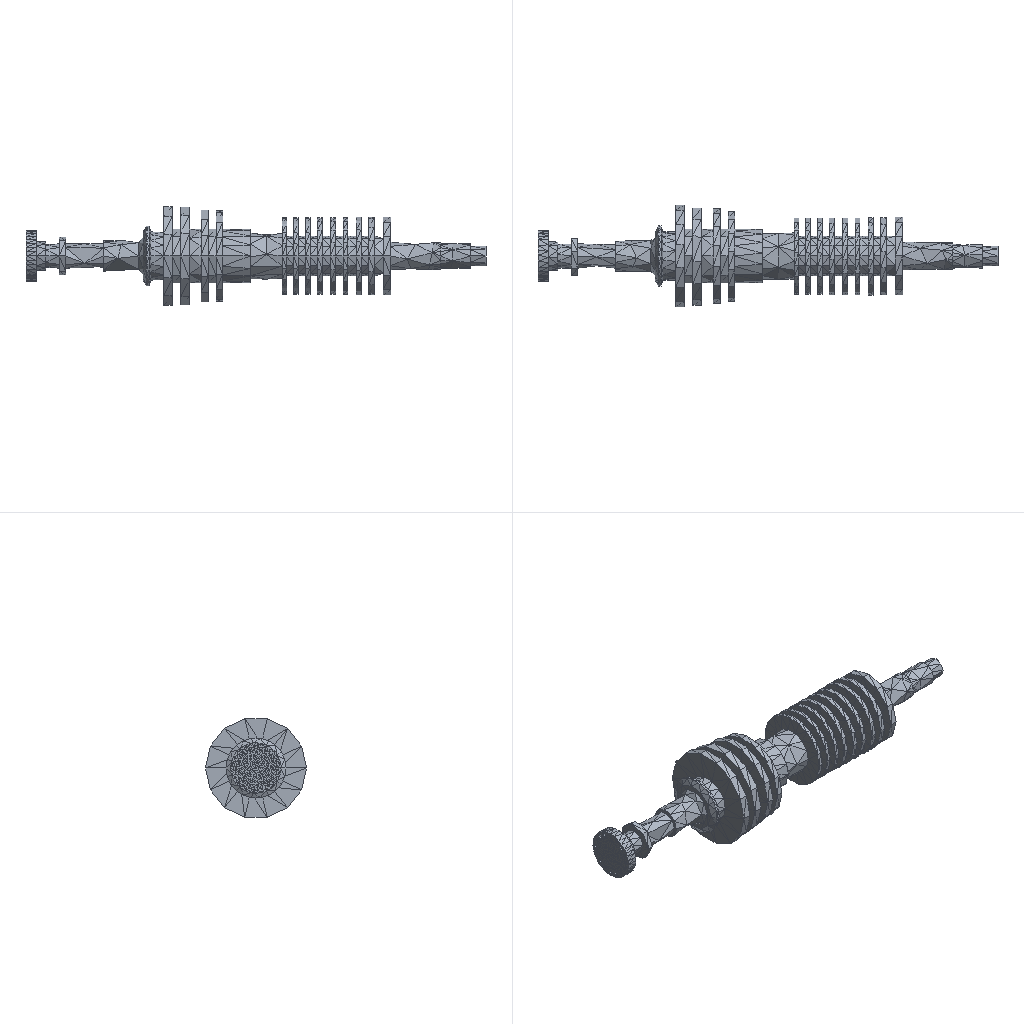Simulation study | ansys workbench
Ansys APDL input file, long lists of numbers shortened:
/batch
/config,noeldb,1     ! force off writing results to database
*get,_wallstrt,active,,time,wall
! ANSYS input file written by Workbench version 2022 R1
! File used for geometry attach:
/title,_______--__ (C5)
! ****** Begin Custom Load Command Snippet ******
/COM, ACT Extensions:
/COM,     LSDYNA, 2021.1
/COM,
! ****** End   Custom Load Command Snippet ******
*DIM,_wb_ProjectScratch_dir,string,248
_wb_ProjectScratch_dir(1) = ''
*DIM,_wb_SolverFiles_dir,string,248
_wb_SolverFiles_dir(1) = ''
*DIM,_wb_userfiles_dir,string,248
_wb_userfiles_dir(1) = ''
/com,--- Data in consistent NMM units. See Solving Units in the help system for more information.
/units,MPA
/nopr
/wb,file,start              !  signify a WB generated input file
/prep7
! Turn off shape checking because checks already performed inside WB mesher.
! See help system for more information.
SHPP,OFF,,NOWARN
/nolist
etcon,set             ! allow ANSYS to choose best KEYOP's for 180x elements, resets any applicable keyopt to MAPDL defaults
/com,*********** Nodes for the whole assembly ***********
nblock,3,,19310
(1i9,3e20.9e3)
        1     4.906201621E+04    -3.060000000E+02     1.550000000E+03
! (17554 more lines like these left out)
-1
/com,*********** Nodes for all Remote Points ***********
nblock,3
(1i9,3e20.9e3)
    17556     4.888853330E+04     3.865628677E-15     1.549999997E+03
-1
/wb,elem,start            !  set before creation of elements
/com,*********** Elements for Body 1 "_____+115mm\_____" ***********
et,1,187
eblock,19,solid,,9763
(19i9)
        1        1        1        1        0        0        0        0       10        0        1     2257     2779     2330     2541    15734    16136    15725    15727
! (19525 more lines like these left out)
-1
/wb,elem,end               !  done creating elements
/com,*********** Send User Defined Coordinate System(s) ***********
csys,0
toffst,273.15,  ! Temperature offset from absolute zero
/com,*********** Set Reference Temperature ***********
tref,22.
/wb,mat,start              !  starting to send materials
/com,*********** Send Materials ***********
Temperature = 'TEMP' ! Temperature
MP,DENS,1,7.85e-09,	! tonne mm^-3
MP,ALPX,1,1.2e-05,	! C^-1
MP,C,1,434000000,	! mm^2 s^-2 C^-1
MP,KXX,1,60.5,	! tonne mm s^-3 C^-1
MP,RSVX,1,0.00017,	! ohm mm
MP,EX,1,200000,	! tonne s^-2 mm^-1
MP,NUXY,1,0.3,
MP,MURX,1,10000,
/wb,mat,end                !  done sending materials
!************************* Model Summary ********************
!_____+115mm\_____,	结构钢,	matid,	1
!************************* End Model Summary ********************
! get the diagonal of the bounding box. Needed later for other things
*get,_xmin,node,,mnloc,x
*get,_ymin,node,,mnloc,y
*get,_zmin,node,,mnloc,z
*get,_xmax,node,,mxloc,x
*get,_ymax,node,,mxloc,y
*get,_zmax,node,,mxloc,z
_ASMDIAG=(_xmax-_xmin)*(_xmax-_xmin)+(_ymax-_ymin)*(_ymax-_ymin)+(_zmax-_zmin)*(_zmax-_zmin)
_ASMDIAG=SQRT(_ASMDIAG)
/wb,contact,start          !  starting to send contact
/wb,contact,end            !  done creating contacts
/golist
/wb,load,start             !  starting to send loads
/com,*********** Fixed Supports ***********
CMBLOCK,_FIXEDSU,NODE,      114
(8i10)
       876       877       878       879       880       881       882       883
! (14 more lines like these left out)
cmsel,s,_FIXEDSU
d,all,all
nsel,all
/com,*********** Create Remote Point "内部远程点" ***********
! -------- Remote Point Used by "力矩" --------
*set,tid,3
*set,cid,2
et,cid,174
et,tid,170
keyo,tid,2,1               ! Don't fix the pilot node
keyo,tid,4,0               ! Activate all DOF's due to large deformation
keyo,cid,12,5              ! Bonded Contact
keyo,cid,4,1               ! Deformable RBE3 style load
keyo,cid,2,2               ! MPC style contact
eblock,10,,,154
(15i9)
    14157        2        2        2        0      857      858     2037     2037     7802     7809     2037     7805
! (153 more lines like these left out)
-1
*set,_npilot,17556
_npilot33=_npilot
type,tid
mat ,cid
real,cid
tshape,pilo
en,14311,_npilot
tshape
/com,*********** Construct Moment Using Remote Attachment ***********
/gst,on,on
fini
*get,_numnode,node,0,count
*get,_numelem,elem,0,count
*get, _MAXELEMNUM, elem, 0, NUM, MAX
*get, _MAXNODENUM, node, 0, NUM, MAX
*get, _MAXELEMTYPE, etyp, 0, NUM, MAX
*get, _MAXREALCONST, real, 0, NUM, MAX
/go
/wb,load,end               !  done creating loads
/com,--- Number of total nodes = %_numnode%
/com,--- Number of contact elements = 154
/com,--- Number of spring elements = 0
/com,--- Number of bearing elements = 0
/com,--- Number of solid elements = 9763
/com,--- Number of condensed parts = 0
/com,--- Number of total elements = %_numelem%
*get,_wallbsol,active,,time,wall
/com,****************************************************************************
/com,*************************    SOLUTION       ********************************
/com,****************************************************************************
/solu
antype,4                   ! transient analysis
nlgeom,on                  ! Turn on Large Deformation Effects
kbc,1                      ! stepped BC's
_thickRatio=  1     ! Ratio of thick parts in the model
eqsl,pcg,1e-8,,,,,,1
cntr,print,1               ! print out contact info and also make no initial contact an error
dmpoption,emat,no             ! Don't combine emat file for DANSYS
dmpoption,esav,no             ! Don't combine esav file for DANSYS
trnopt,full,,,,,hht        ! HHT time integration method
tintp, mosp			! Choose transient integration settings for moderate speed application
nldiag,cont,iter           ! print out contact info each equilibrium iteration
rescontrol,define,last,last,,dele	   ! Program Controlled
/com,****************************************************
/com,******************* SOLVE FOR LS 1 OF 1 ****************
nsel,s,node,,17556
f,all,mx,150.
f,all,my,0.
f,all,mz,0.
nsel,all
/nopr
/gopr
autots,on                   ! User turned on automatic time stepping
deltim,20,20,20,OFF
time,20.
timint,on                  ! Turn on time integration effects
outres,erase
outres,all,none
outres,nsol,all,
outres,rsol,all
outres,eangl,all
outres,etmp,all
outres,veng,all
outres,strs,all,
outres,epel,all,
outres,eppl,all,
outres,cont,all,
outres,v,all,
outres,a,all,
! *********** WB SOLVE COMMAND ***********
! check interactive state
*get,ANSINTER_,active,,int
*if,ANSINTER_,ne,0,then
/eof
*endif
solve
/com *************** Write FE CONNECTORS *********
CEWRITE,file,ce,,INTE
/com,****************************************************
/com,*************** FINISHED SOLVE FOR LS 1 *************
*get,_wallasol,active,,time,wall
/nopr
*get,_numnode,node,0,count
*get,_numelem,elem,0,count
*get, _MAXELEMNUM, elem, 0, NUM, MAX
*get, _MAXNODENUM, node, 0, NUM, MAX,,,INTERNAL
*get, _MAXELEMTYPE, etyp, 0, NUM, MAX
*get, _MAXREALCONST, real, 0, NUM, MAX
/gopr
*get,_PCGITER,active,,solu,cgiter
/post1
xmlo,ENCODING,ISO-8859-1
xmlo,parm
/xml,parm,xml
fini
/gopr
*get,_walldone,active,,time,wall
_preptime=(_wallbsol-_wallstrt)*3600
_solvtime=(_wallasol-_wallbsol)*3600
_posttime=(_walldone-_wallasol)*3600
_totaltim=(_walldone-_wallstrt)*3600
*get,_dlbratio,active,0,solu,dlbr
*get,_combtime,active,0,solu,comb
*get,_ssmode,active,0,solu,ssmm
*get,_ndofs,active,0,solu,ndof
*get,_sol_end_time,active,0,set,time
*if,_sol_end_time,eq,20.,then
/fclean				!clean distributed files
*endif
/com,--- Total number of nodes = %_numnode%
/com,--- Total number of elements = %_numelem%
/com,--- Element load balance ratio = %_dlbratio%
/com,--- Time to combine distributed files = %_combtime%
/com,--- Sparse memory mode = %_ssmode%
/com,--- Number of DOF = %_ndofs%
/wb,file,end               ! done with WB generated input